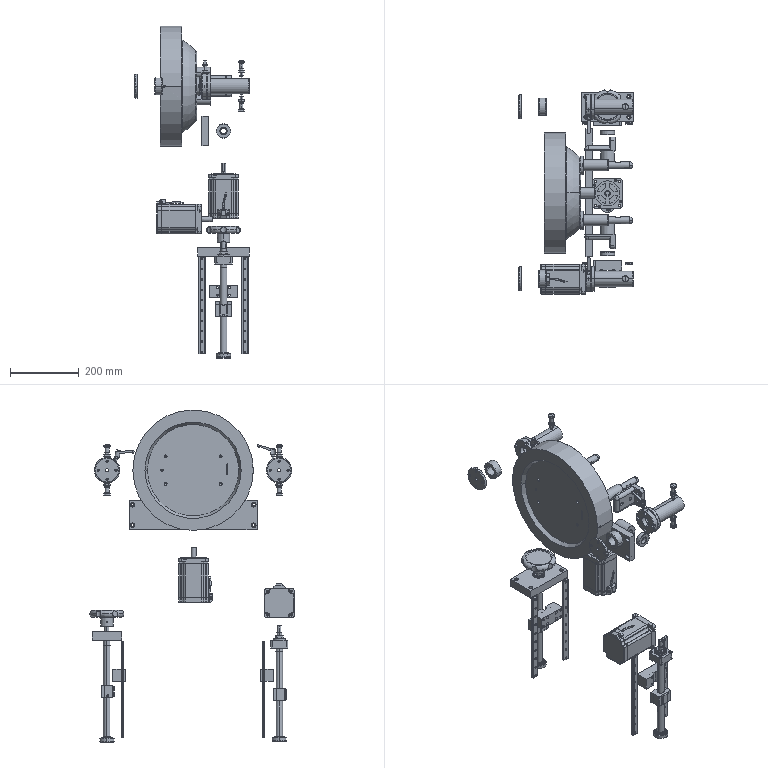Part | NX | features BREP 43 | 72 solids | 5562 faces | volume 11833919 mm3 | cylinder 2772 | plane 1695 | torus 392 | cone 366 | sphere 254 | spline 83 | commonest cylinder face diameters 0.1 x896 18 x364 17.4 x360 6.5 x108 10 x92 3.5 x80